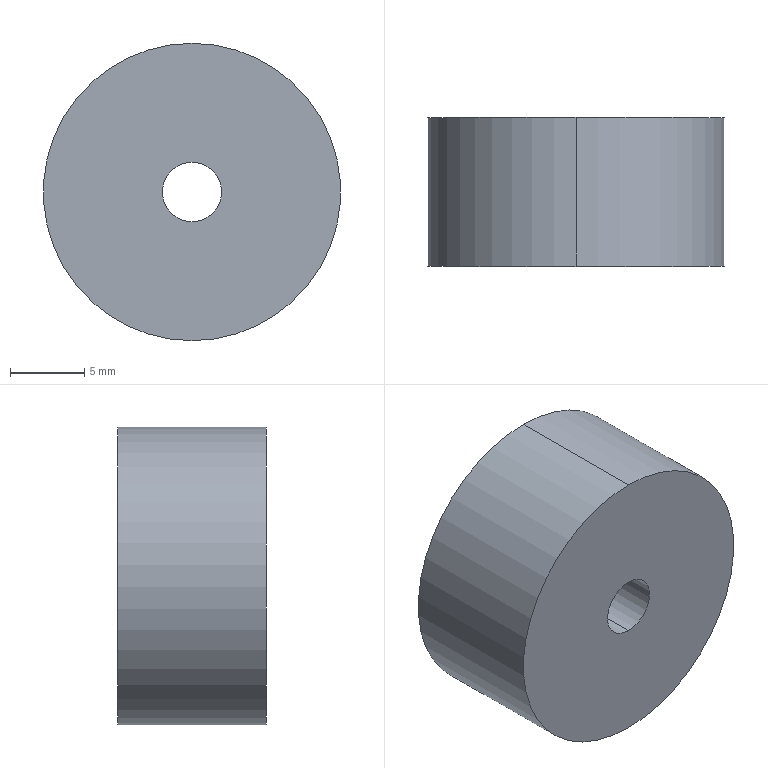Part | STEP file | 1 solid | 9 faces | box 20 x 10 x 20 mm | volume 2790 mm3 | cylinder 6 | plane 3 | commonest cylinder face diameters 4 x2 8 x2 20 x2
STEP:
#1=CARTESIAN_POINT('',(0.,0.,0.));
#2=DIRECTION('',(0.,0.,1.));
#3=DIRECTION('',(1.,0.,0.));
#4=AXIS2_PLACEMENT_3D('',#1,#2,#3);
#5=CARTESIAN_POINT('',(0.,4.,4.));
#6=VERTEX_POINT('',#5);
#7=CARTESIAN_POINT('',(0.,10.,4.));
#8=VERTEX_POINT('',#7);
#9=CARTESIAN_POINT('',(0.,10.,4.));
#10=DIRECTION('',(0.,1.,0.));
#11=VECTOR('',#10,1.);
#12=LINE('',#9,#11);
#13=CARTESIAN_POINT('',(0.,10.,0.));
#14=DIRECTION('',(0.,1.,0.));
#15=DIRECTION('',(0.,0.,1.));
#16=AXIS2_PLACEMENT_3D('',#13,#14,#15);
#17=CYLINDRICAL_SURFACE('',#16,4.);
#18=CARTESIAN_POINT('',(6.283,0.));
#19=DIRECTION('',(0.,1.));
#20=VECTOR('',#19,1.);
#21=LINE('',#18,#20);
#22=(GEOMETRIC_REPRESENTATION_CONTEXT(2)PARAMETRIC_REPRESENTATION_CONTEXT()REPRESENTATION_CONTEXT('',''));
#23=DEFINITIONAL_REPRESENTATION('',(#21),#22);
#24=PCURVE('',#17,#23);
#25=CARTESIAN_POINT('',(0.,10.,0.));
#26=DIRECTION('',(0.,1.,0.));
#27=DIRECTION('',(0.,0.,1.));
#28=AXIS2_PLACEMENT_3D('',#25,#26,#27);
#29=CYLINDRICAL_SURFACE('',#28,4.);
#30=CARTESIAN_POINT('',(0.,0.));
#31=DIRECTION('',(0.,1.));
#32=VECTOR('',#31,1.);
#33=LINE('',#30,#32);
#34=(GEOMETRIC_REPRESENTATION_CONTEXT(2)PARAMETRIC_REPRESENTATION_CONTEXT()REPRESENTATION_CONTEXT('',''));
#35=DEFINITIONAL_REPRESENTATION('',(#33),#34);
#36=PCURVE('',#29,#35);
#37=SURFACE_CURVE('',#12,(#24,#36),.PCURVE_S1.);
#38=EDGE_CURVE('',#6,#8,#37,.T.);
#39=ORIENTED_EDGE('',*,*,#38,.T.);
#40=CARTESIAN_POINT('',(0.,10.,-4.));
#41=VERTEX_POINT('',#40);
#42=CARTESIAN_POINT('',(0.,10.,0.));
#43=DIRECTION('',(0.,1.,0.));
#44=DIRECTION('',(0.,0.,1.));
#45=AXIS2_PLACEMENT_3D('',#42,#43,#44);
#46=CIRCLE('',#45,4.);
#47=CARTESIAN_POINT('',(0.,0.));
#48=DIRECTION('',(1.,0.));
#49=VECTOR('',#48,1.);
#50=LINE('',#47,#49);
#51=(GEOMETRIC_REPRESENTATION_CONTEXT(2)PARAMETRIC_REPRESENTATION_CONTEXT()REPRESENTATION_CONTEXT('',''));
#52=DEFINITIONAL_REPRESENTATION('',(#50),#51);
#53=PCURVE('',#17,#52);
#54=CARTESIAN_POINT('',(0.,10.,0.));
#55=DIRECTION('',(0.,1.,0.));
#56=DIRECTION('',(0.,0.,1.));
#57=AXIS2_PLACEMENT_3D('',#54,#55,#56);
#58=PLANE('',#57);
#59=CARTESIAN_POINT('',(0.,0.));
#60=DIRECTION('',(1.,0.));
#61=AXIS2_PLACEMENT_2D('',#59,#60);
#62=CIRCLE('',#61,4.);
#63=(GEOMETRIC_REPRESENTATION_CONTEXT(2)PARAMETRIC_REPRESENTATION_CONTEXT()REPRESENTATION_CONTEXT('',''));
#64=DEFINITIONAL_REPRESENTATION('',(#62),#63);
#65=PCURVE('',#58,#64);
#66=SURFACE_CURVE('',#46,(#53,#65),.PCURVE_S1.);
#67=EDGE_CURVE('',#41,#8,#66,.T.);
#68=ORIENTED_EDGE('',*,*,#67,.F.);
#69=CARTESIAN_POINT('',(0.,4.,-4.));
#70=VERTEX_POINT('',#69);
#71=CARTESIAN_POINT('',(0.,10.,-4.));
#72=DIRECTION('',(0.,1.,0.));
#73=VECTOR('',#72,1.);
#74=LINE('',#71,#73);
#75=CARTESIAN_POINT('',(3.142,0.));
#76=DIRECTION('',(0.,1.));
#77=VECTOR('',#76,1.);
#78=LINE('',#75,#77);
#79=(GEOMETRIC_REPRESENTATION_CONTEXT(2)PARAMETRIC_REPRESENTATION_CONTEXT()REPRESENTATION_CONTEXT('',''));
#80=DEFINITIONAL_REPRESENTATION('',(#78),#79);
#81=PCURVE('',#17,#80);
#82=CARTESIAN_POINT('',(3.142,0.));
#83=DIRECTION('',(0.,1.));
#84=VECTOR('',#83,1.);
#85=LINE('',#82,#84);
#86=(GEOMETRIC_REPRESENTATION_CONTEXT(2)PARAMETRIC_REPRESENTATION_CONTEXT()REPRESENTATION_CONTEXT('',''));
#87=DEFINITIONAL_REPRESENTATION('',(#85),#86);
#88=PCURVE('',#29,#87);
#89=SURFACE_CURVE('',#74,(#81,#88),.PCURVE_S1.);
#90=EDGE_CURVE('',#70,#41,#89,.T.);
#91=ORIENTED_EDGE('',*,*,#90,.F.);
#92=CARTESIAN_POINT('',(0.,4.,0.));
#93=DIRECTION('',(0.,1.,0.));
#94=DIRECTION('',(0.,0.,1.));
#95=AXIS2_PLACEMENT_3D('',#92,#93,#94);
#96=CIRCLE('',#95,4.);
#97=CARTESIAN_POINT('',(0.,-6.));
#98=DIRECTION('',(1.,0.));
#99=VECTOR('',#98,1.);
#100=LINE('',#97,#99);
#101=(GEOMETRIC_REPRESENTATION_CONTEXT(2)PARAMETRIC_REPRESENTATION_CONTEXT()REPRESENTATION_CONTEXT('',''));
#102=DEFINITIONAL_REPRESENTATION('',(#100),#101);
#103=PCURVE('',#17,#102);
#104=CARTESIAN_POINT('',(2.,4.,0.));
#105=DIRECTION('',(0.,-1.,0.));
#106=DIRECTION('',(0.,0.,-1.));
#107=AXIS2_PLACEMENT_3D('',#104,#105,#106);
#108=PLANE('',#107);
#109=CARTESIAN_POINT('',(-4.,-2.));
#110=CARTESIAN_POINT('',(-4.,4.928));
#111=CARTESIAN_POINT('',(2.,1.464));
#112=CARTESIAN_POINT('',(8.,-2.));
#113=CARTESIAN_POINT('',(2.,-5.464));
#114=CARTESIAN_POINT('',(-4.,-8.928));
#115=CARTESIAN_POINT('',(-4.,-2.));
#116=(BOUNDED_CURVE()B_SPLINE_CURVE(2,(#109,#110,#111,#112,#113,#114,#115),.UNSPECIFIED.,.T.,.F.)B_SPLINE_CURVE_WITH_KNOTS((1,2,2,2,2,1),(-2.094,0.,2.094,4.189,6.283,8.378),.UNSPECIFIED.)CURVE()GEOMETRIC_REPRESENTATION_ITEM()RATIONAL_B_SPLINE_CURVE((1.,0.5,1.,0.5,1.,0.5,1.))REPRESENTATION_ITEM(''));
#117=(GEOMETRIC_REPRESENTATION_CONTEXT(2)PARAMETRIC_REPRESENTATION_CONTEXT()REPRESENTATION_CONTEXT('',''));
#118=DEFINITIONAL_REPRESENTATION('',(#116),#117);
#119=PCURVE('',#108,#118);
#120=SURFACE_CURVE('',#96,(#103,#119),.PCURVE_S1.);
#121=EDGE_CURVE('',#70,#6,#120,.T.);
#122=ORIENTED_EDGE('',*,*,#121,.T.);
#123=EDGE_LOOP('',(#39,#68,#91,#122));
#124=FACE_BOUND('',#123,.F.);
#125=ADVANCED_FACE('',(#124),#17,.F.);
#126=CARTESIAN_POINT('',(0.,0.,2.));
#127=VERTEX_POINT('',#126);
#128=CARTESIAN_POINT('',(0.,4.,2.));
#129=VERTEX_POINT('',#128);
#130=CARTESIAN_POINT('',(0.,10.,2.));
#131=DIRECTION('',(0.,1.,0.));
#132=VECTOR('',#131,1.);
#133=LINE('',#130,#132);
#134=CARTESIAN_POINT('',(0.,10.,0.));
#135=DIRECTION('',(0.,1.,0.));
#136=DIRECTION('',(0.,0.,1.));
#137=AXIS2_PLACEMENT_3D('',#134,#135,#136);
#138=CYLINDRICAL_SURFACE('',#137,2.);
#139=CARTESIAN_POINT('',(6.283,0.));
#140=DIRECTION('',(0.,1.));
#141=VECTOR('',#140,1.);
#142=LINE('',#139,#141);
#143=(GEOMETRIC_REPRESENTATION_CONTEXT(2)PARAMETRIC_REPRESENTATION_CONTEXT()REPRESENTATION_CONTEXT('',''));
#144=DEFINITIONAL_REPRESENTATION('',(#142),#143);
#145=PCURVE('',#138,#144);
#146=CARTESIAN_POINT('',(0.,10.,0.));
#147=DIRECTION('',(0.,1.,0.));
#148=DIRECTION('',(0.,0.,1.));
#149=AXIS2_PLACEMENT_3D('',#146,#147,#148);
#150=CYLINDRICAL_SURFACE('',#149,2.);
#151=CARTESIAN_POINT('',(0.,0.));
#152=DIRECTION('',(0.,1.));
#153=VECTOR('',#152,1.);
#154=LINE('',#151,#153);
#155=(GEOMETRIC_REPRESENTATION_CONTEXT(2)PARAMETRIC_REPRESENTATION_CONTEXT()REPRESENTATION_CONTEXT('',''));
#156=DEFINITIONAL_REPRESENTATION('',(#154),#155);
#157=PCURVE('',#150,#156);
#158=SURFACE_CURVE('',#133,(#145,#157),.PCURVE_S1.);
#159=EDGE_CURVE('',#127,#129,#158,.T.);
#160=ORIENTED_EDGE('',*,*,#159,.T.);
#161=CARTESIAN_POINT('',(0.,4.,-2.));
#162=VERTEX_POINT('',#161);
#163=CARTESIAN_POINT('',(0.,4.,0.));
#164=DIRECTION('',(0.,1.,0.));
#165=DIRECTION('',(0.,0.,1.));
#166=AXIS2_PLACEMENT_3D('',#163,#164,#165);
#167=CIRCLE('',#166,2.);
#168=CARTESIAN_POINT('',(0.,-6.));
#169=DIRECTION('',(1.,0.));
#170=VECTOR('',#169,1.);
#171=LINE('',#168,#170);
#172=(GEOMETRIC_REPRESENTATION_CONTEXT(2)PARAMETRIC_REPRESENTATION_CONTEXT()REPRESENTATION_CONTEXT('',''));
#173=DEFINITIONAL_REPRESENTATION('',(#171),#172);
#174=PCURVE('',#138,#173);
#175=CARTESIAN_POINT('',(-2.,-2.));
#176=CARTESIAN_POINT('',(-2.,1.464));
#177=CARTESIAN_POINT('',(1.,-0.2679));
#178=CARTESIAN_POINT('',(4.,-2.));
#179=CARTESIAN_POINT('',(1.,-3.732));
#180=CARTESIAN_POINT('',(-2.,-5.464));
#181=CARTESIAN_POINT('',(-2.,-2.));
#182=(BOUNDED_CURVE()B_SPLINE_CURVE(2,(#175,#176,#177,#178,#179,#180,#181),.UNSPECIFIED.,.T.,.F.)B_SPLINE_CURVE_WITH_KNOTS((1,2,2,2,2,1),(-2.094,0.,2.094,4.189,6.283,8.378),.UNSPECIFIED.)CURVE()GEOMETRIC_REPRESENTATION_ITEM()RATIONAL_B_SPLINE_CURVE((1.,0.5,1.,0.5,1.,0.5,1.))REPRESENTATION_ITEM(''));
#183=(GEOMETRIC_REPRESENTATION_CONTEXT(2)PARAMETRIC_REPRESENTATION_CONTEXT()REPRESENTATION_CONTEXT('',''));
#184=DEFINITIONAL_REPRESENTATION('',(#182),#183);
#185=PCURVE('',#108,#184);
#186=SURFACE_CURVE('',#167,(#174,#185),.PCURVE_S1.);
#187=EDGE_CURVE('',#162,#129,#186,.T.);
#188=ORIENTED_EDGE('',*,*,#187,.F.);
#189=CARTESIAN_POINT('',(0.,0.,-2.));
#190=VERTEX_POINT('',#189);
#191=CARTESIAN_POINT('',(0.,10.,-2.));
#192=DIRECTION('',(0.,1.,0.));
#193=VECTOR('',#192,1.);
#194=LINE('',#191,#193);
#195=CARTESIAN_POINT('',(3.142,0.));
#196=DIRECTION('',(0.,1.));
#197=VECTOR('',#196,1.);
#198=LINE('',#195,#197);
#199=(GEOMETRIC_REPRESENTATION_CONTEXT(2)PARAMETRIC_REPRESENTATION_CONTEXT()REPRESENTATION_CONTEXT('',''));
#200=DEFINITIONAL_REPRESENTATION('',(#198),#199);
#201=PCURVE('',#138,#200);
#202=CARTESIAN_POINT('',(3.142,0.));
#203=DIRECTION('',(0.,1.));
#204=VECTOR('',#203,1.);
#205=LINE('',#202,#204);
#206=(GEOMETRIC_REPRESENTATION_CONTEXT(2)PARAMETRIC_REPRESENTATION_CONTEXT()REPRESENTATION_CONTEXT('',''));
#207=DEFINITIONAL_REPRESENTATION('',(#205),#206);
#208=PCURVE('',#150,#207);
#209=SURFACE_CURVE('',#194,(#201,#208),.PCURVE_S1.);
#210=EDGE_CURVE('',#190,#162,#209,.T.);
#211=ORIENTED_EDGE('',*,*,#210,.F.);
#212=CARTESIAN_POINT('',(0.,0.,0.));
#213=DIRECTION('',(0.,1.,0.));
#214=DIRECTION('',(0.,0.,1.));
#215=AXIS2_PLACEMENT_3D('',#212,#213,#214);
#216=CIRCLE('',#215,2.);
#217=CARTESIAN_POINT('',(0.,-10.));
#218=DIRECTION('',(1.,0.));
#219=VECTOR('',#218,1.);
#220=LINE('',#217,#219);
#221=(GEOMETRIC_REPRESENTATION_CONTEXT(2)PARAMETRIC_REPRESENTATION_CONTEXT()REPRESENTATION_CONTEXT('',''));
#222=DEFINITIONAL_REPRESENTATION('',(#220),#221);
#223=PCURVE('',#138,#222);
#224=CARTESIAN_POINT('',(0.,0.,0.));
#225=DIRECTION('',(0.,1.,0.));
#226=DIRECTION('',(0.,0.,1.));
#227=AXIS2_PLACEMENT_3D('',#224,#225,#226);
#228=PLANE('',#227);
#229=CARTESIAN_POINT('',(0.,0.));
#230=DIRECTION('',(1.,0.));
#231=AXIS2_PLACEMENT_2D('',#229,#230);
#232=CIRCLE('',#231,2.);
#233=(GEOMETRIC_REPRESENTATION_CONTEXT(2)PARAMETRIC_REPRESENTATION_CONTEXT()REPRESENTATION_CONTEXT('',''));
#234=DEFINITIONAL_REPRESENTATION('',(#232),#233);
#235=PCURVE('',#228,#234);
#236=SURFACE_CURVE('',#216,(#223,#235),.PCURVE_S1.);
#237=EDGE_CURVE('',#190,#127,#236,.T.);
#238=ORIENTED_EDGE('',*,*,#237,.T.);
#239=EDGE_LOOP('',(#160,#188,#211,#238));
#240=FACE_BOUND('',#239,.F.);
#241=ADVANCED_FACE('',(#240),#138,.F.);
#242=CARTESIAN_POINT('',(0.,10.,10.));
#243=VERTEX_POINT('',#242);
#244=CARTESIAN_POINT('',(0.,10.,-10.));
#245=VERTEX_POINT('',#244);
#246=CARTESIAN_POINT('',(0.,10.,0.));
#247=DIRECTION('',(0.,1.,0.));
#248=DIRECTION('',(0.,0.,1.));
#249=AXIS2_PLACEMENT_3D('',#246,#247,#248);
#250=CIRCLE('',#249,10.);
#251=CARTESIAN_POINT('',(0.,10.,0.));
#252=DIRECTION('',(0.,-1.,0.));
#253=DIRECTION('',(0.,0.,-1.));
#254=AXIS2_PLACEMENT_3D('',#251,#252,#253);
#255=CYLINDRICAL_SURFACE('',#254,10.);
#256=CARTESIAN_POINT('',(3.142,0.));
#257=DIRECTION('',(-1.,0.));
#258=VECTOR('',#257,1.);
#259=LINE('',#256,#258);
#260=(GEOMETRIC_REPRESENTATION_CONTEXT(2)PARAMETRIC_REPRESENTATION_CONTEXT()REPRESENTATION_CONTEXT('',''));
#261=DEFINITIONAL_REPRESENTATION('',(#259),#260);
#262=PCURVE('',#255,#261);
#263=CARTESIAN_POINT('',(0.,0.));
#264=DIRECTION('',(1.,0.));
#265=AXIS2_PLACEMENT_2D('',#263,#264);
#266=CIRCLE('',#265,10.);
#267=(GEOMETRIC_REPRESENTATION_CONTEXT(2)PARAMETRIC_REPRESENTATION_CONTEXT()REPRESENTATION_CONTEXT('',''));
#268=DEFINITIONAL_REPRESENTATION('',(#266),#267);
#269=PCURVE('',#58,#268);
#270=SURFACE_CURVE('',#250,(#262,#269),.PCURVE_S1.);
#271=EDGE_CURVE('',#243,#245,#270,.T.);
#272=ORIENTED_EDGE('',*,*,#271,.F.);
#273=CARTESIAN_POINT('',(0.,0.,10.));
#274=VERTEX_POINT('',#273);
#275=CARTESIAN_POINT('',(0.,10.,10.));
#276=DIRECTION('',(0.,-1.,0.));
#277=VECTOR('',#276,1.);
#278=LINE('',#275,#277);
#279=CARTESIAN_POINT('',(3.142,0.));
#280=DIRECTION('',(0.,1.));
#281=VECTOR('',#280,1.);
#282=LINE('',#279,#281);
#283=(GEOMETRIC_REPRESENTATION_CONTEXT(2)PARAMETRIC_REPRESENTATION_CONTEXT()REPRESENTATION_CONTEXT('',''));
#284=DEFINITIONAL_REPRESENTATION('',(#282),#283);
#285=PCURVE('',#255,#284);
#286=CARTESIAN_POINT('',(0.,10.,0.));
#287=DIRECTION('',(0.,-1.,0.));
#288=DIRECTION('',(0.,0.,-1.));
#289=AXIS2_PLACEMENT_3D('',#286,#287,#288);
#290=CYLINDRICAL_SURFACE('',#289,10.);
#291=CARTESIAN_POINT('',(3.142,0.));
#292=DIRECTION('',(0.,1.));
#293=VECTOR('',#292,1.);
#294=LINE('',#291,#293);
#295=(GEOMETRIC_REPRESENTATION_CONTEXT(2)PARAMETRIC_REPRESENTATION_CONTEXT()REPRESENTATION_CONTEXT('',''));
#296=DEFINITIONAL_REPRESENTATION('',(#294),#295);
#297=PCURVE('',#290,#296);
#298=SURFACE_CURVE('',#278,(#285,#297),.PCURVE_S1.);
#299=EDGE_CURVE('',#243,#274,#298,.T.);
#300=ORIENTED_EDGE('',*,*,#299,.T.);
#301=CARTESIAN_POINT('',(0.,0.,-10.));
#302=VERTEX_POINT('',#301);
#303=CARTESIAN_POINT('',(0.,0.,0.));
#304=DIRECTION('',(0.,1.,0.));
#305=DIRECTION('',(0.,0.,1.));
#306=AXIS2_PLACEMENT_3D('',#303,#304,#305);
#307=CIRCLE('',#306,10.);
#308=CARTESIAN_POINT('',(3.142,10.));
#309=DIRECTION('',(-1.,0.));
#310=VECTOR('',#309,1.);
#311=LINE('',#308,#310);
#312=(GEOMETRIC_REPRESENTATION_CONTEXT(2)PARAMETRIC_REPRESENTATION_CONTEXT()REPRESENTATION_CONTEXT('',''));
#313=DEFINITIONAL_REPRESENTATION('',(#311),#312);
#314=PCURVE('',#255,#313);
#315=CARTESIAN_POINT('',(0.,0.));
#316=DIRECTION('',(1.,0.));
#317=AXIS2_PLACEMENT_2D('',#315,#316);
#318=CIRCLE('',#317,10.);
#319=(GEOMETRIC_REPRESENTATION_CONTEXT(2)PARAMETRIC_REPRESENTATION_CONTEXT()REPRESENTATION_CONTEXT('',''));
#320=DEFINITIONAL_REPRESENTATION('',(#318),#319);
#321=PCURVE('',#228,#320);
#322=SURFACE_CURVE('',#307,(#314,#321),.PCURVE_S1.);
#323=EDGE_CURVE('',#274,#302,#322,.T.);
#324=ORIENTED_EDGE('',*,*,#323,.T.);
#325=CARTESIAN_POINT('',(0.,10.,-10.));
#326=DIRECTION('',(0.,-1.,0.));
#327=VECTOR('',#326,1.);
#328=LINE('',#325,#327);
#329=CARTESIAN_POINT('',(0.,0.));
#330=DIRECTION('',(0.,1.));
#331=VECTOR('',#330,1.);
#332=LINE('',#329,#331);
#333=(GEOMETRIC_REPRESENTATION_CONTEXT(2)PARAMETRIC_REPRESENTATION_CONTEXT()REPRESENTATION_CONTEXT('',''));
#334=DEFINITIONAL_REPRESENTATION('',(#332),#333);
#335=PCURVE('',#255,#334);
#336=CARTESIAN_POINT('',(6.283,0.));
#337=DIRECTION('',(0.,1.));
#338=VECTOR('',#337,1.);
#339=LINE('',#336,#338);
#340=(GEOMETRIC_REPRESENTATION_CONTEXT(2)PARAMETRIC_REPRESENTATION_CONTEXT()REPRESENTATION_CONTEXT('',''));
#341=DEFINITIONAL_REPRESENTATION('',(#339),#340);
#342=PCURVE('',#290,#341);
#343=SURFACE_CURVE('',#328,(#335,#342),.PCURVE_S1.);
#344=EDGE_CURVE('',#245,#302,#343,.T.);
#345=ORIENTED_EDGE('',*,*,#344,.F.);
#346=EDGE_LOOP('',(#272,#300,#324,#345));
#347=FACE_BOUND('',#346,.T.);
#348=ADVANCED_FACE('',(#347),#255,.T.);
#349=ORIENTED_EDGE('',*,*,#299,.F.);
#350=CARTESIAN_POINT('',(0.,10.,0.));
#351=DIRECTION('',(0.,1.,0.));
#352=DIRECTION('',(0.,0.,1.));
#353=AXIS2_PLACEMENT_3D('',#350,#351,#352);
#354=CIRCLE('',#353,10.);
#355=CARTESIAN_POINT('',(9.425,0.));
#356=DIRECTION('',(-1.,0.));
#357=VECTOR('',#356,1.);
#358=LINE('',#355,#357);
#359=(GEOMETRIC_REPRESENTATION_CONTEXT(2)PARAMETRIC_REPRESENTATION_CONTEXT()REPRESENTATION_CONTEXT('',''));
#360=DEFINITIONAL_REPRESENTATION('',(#358),#359);
#361=PCURVE('',#290,#360);
#362=CARTESIAN_POINT('',(0.,0.));
#363=DIRECTION('',(1.,0.));
#364=AXIS2_PLACEMENT_2D('',#362,#363);
#365=CIRCLE('',#364,10.);
#366=(GEOMETRIC_REPRESENTATION_CONTEXT(2)PARAMETRIC_REPRESENTATION_CONTEXT()REPRESENTATION_CONTEXT('',''));
#367=DEFINITIONAL_REPRESENTATION('',(#365),#366);
#368=PCURVE('',#58,#367);
#369=SURFACE_CURVE('',#354,(#361,#368),.PCURVE_S1.);
#370=EDGE_CURVE('',#245,#243,#369,.T.);
#371=ORIENTED_EDGE('',*,*,#370,.F.);
#372=ORIENTED_EDGE('',*,*,#344,.T.);
#373=CARTESIAN_POINT('',(0.,0.,0.));
#374=DIRECTION('',(0.,1.,0.));
#375=DIRECTION('',(0.,0.,1.));
#376=AXIS2_PLACEMENT_3D('',#373,#374,#375);
#377=CIRCLE('',#376,10.);
#378=CARTESIAN_POINT('',(9.425,10.));
#379=DIRECTION('',(-1.,0.));
#380=VECTOR('',#379,1.);
#381=LINE('',#378,#380);
#382=(GEOMETRIC_REPRESENTATION_CONTEXT(2)PARAMETRIC_REPRESENTATION_CONTEXT()REPRESENTATION_CONTEXT('',''));
#383=DEFINITIONAL_REPRESENTATION('',(#381),#382);
#384=PCURVE('',#290,#383);
#385=CARTESIAN_POINT('',(0.,0.));
#386=DIRECTION('',(1.,0.));
#387=AXIS2_PLACEMENT_2D('',#385,#386);
#388=CIRCLE('',#387,10.);
#389=(GEOMETRIC_REPRESENTATION_CONTEXT(2)PARAMETRIC_REPRESENTATION_CONTEXT()REPRESENTATION_CONTEXT('',''));
#390=DEFINITIONAL_REPRESENTATION('',(#388),#389);
#391=PCURVE('',#228,#390);
#392=SURFACE_CURVE('',#377,(#384,#391),.PCURVE_S1.);
#393=EDGE_CURVE('',#302,#274,#392,.T.);
#394=ORIENTED_EDGE('',*,*,#393,.T.);
#395=EDGE_LOOP('',(#349,#371,#372,#394));
#396=FACE_BOUND('',#395,.T.);
#397=ADVANCED_FACE('',(#396),#290,.T.);
#398=CARTESIAN_POINT('',(0.,10.,0.));
#399=DIRECTION('',(0.,1.,0.));
#400=DIRECTION('',(0.,0.,1.));
#401=AXIS2_PLACEMENT_3D('',#398,#399,#400);
#402=CIRCLE('',#401,4.);
#403=CARTESIAN_POINT('',(0.,0.));
#404=DIRECTION('',(1.,0.));
#405=AXIS2_PLACEMENT_2D('',#403,#404);
#406=CIRCLE('',#405,4.);
#407=(GEOMETRIC_REPRESENTATION_CONTEXT(2)PARAMETRIC_REPRESENTATION_CONTEXT()REPRESENTATION_CONTEXT('',''));
#408=DEFINITIONAL_REPRESENTATION('',(#406),#407);
#409=PCURVE('',#58,#408);
#410=CARTESIAN_POINT('',(0.,0.));
#411=DIRECTION('',(1.,0.));
#412=VECTOR('',#411,1.);
#413=LINE('',#410,#412);
#414=(GEOMETRIC_REPRESENTATION_CONTEXT(2)PARAMETRIC_REPRESENTATION_CONTEXT()REPRESENTATION_CONTEXT('',''));
#415=DEFINITIONAL_REPRESENTATION('',(#413),#414);
#416=PCURVE('',#29,#415);
#417=SURFACE_CURVE('',#402,(#409,#416),.PCURVE_S1.);
#418=EDGE_CURVE('',#8,#41,#417,.T.);
#419=ORIENTED_EDGE('',*,*,#418,.F.);
#420=ORIENTED_EDGE('',*,*,#67,.F.);
#421=EDGE_LOOP('',(#419,#420));
#422=FACE_BOUND('',#421,.T.);
#423=ORIENTED_EDGE('',*,*,#370,.T.);
#424=ORIENTED_EDGE('',*,*,#271,.T.);
#425=EDGE_LOOP('',(#423,#424));
#426=FACE_BOUND('',#425,.T.);
#427=ADVANCED_FACE('',(#422,#426),#58,.T.);
#428=CARTESIAN_POINT('',(0.,0.,0.));
#429=DIRECTION('',(0.,1.,0.));
#430=DIRECTION('',(0.,0.,1.));
#431=AXIS2_PLACEMENT_3D('',#428,#429,#430);
#432=CIRCLE('',#431,2.);
#433=CARTESIAN_POINT('',(0.,0.));
#434=DIRECTION('',(1.,0.));
#435=AXIS2_PLACEMENT_2D('',#433,#434);
#436=CIRCLE('',#435,2.);
#437=(GEOMETRIC_REPRESENTATION_CONTEXT(2)PARAMETRIC_REPRESENTATION_CONTEXT()REPRESENTATION_CONTEXT('',''));
#438=DEFINITIONAL_REPRESENTATION('',(#436),#437);
#439=PCURVE('',#228,#438);
#440=CARTESIAN_POINT('',(0.,-10.));
#441=DIRECTION('',(1.,0.));
#442=VECTOR('',#441,1.);
#443=LINE('',#440,#442);
#444=(GEOMETRIC_REPRESENTATION_CONTEXT(2)PARAMETRIC_REPRESENTATION_CONTEXT()REPRESENTATION_CONTEXT('',''));
#445=DEFINITIONAL_REPRESENTATION('',(#443),#444);
#446=PCURVE('',#150,#445);
#447=SURFACE_CURVE('',#432,(#439,#446),.PCURVE_S1.);
#448=EDGE_CURVE('',#127,#190,#447,.T.);
#449=ORIENTED_EDGE('',*,*,#448,.T.);
#450=ORIENTED_EDGE('',*,*,#237,.T.);
#451=EDGE_LOOP('',(#449,#450));
#452=FACE_BOUND('',#451,.T.);
#453=ORIENTED_EDGE('',*,*,#393,.F.);
#454=ORIENTED_EDGE('',*,*,#323,.F.);
#455=EDGE_LOOP('',(#453,#454));
#456=FACE_BOUND('',#455,.T.);
#457=ADVANCED_FACE('',(#452,#456),#228,.F.);
#458=CARTESIAN_POINT('',(0.,4.,0.));
#459=DIRECTION('',(0.,1.,0.));
#460=DIRECTION('',(0.,0.,1.));
#461=AXIS2_PLACEMENT_3D('',#458,#459,#460);
#462=CIRCLE('',#461,2.);
#463=CARTESIAN_POINT('',(0.,-6.));
#464=DIRECTION('',(1.,0.));
#465=VECTOR('',#464,1.);
#466=LINE('',#463,#465);
#467=(GEOMETRIC_REPRESENTATION_CONTEXT(2)PARAMETRIC_REPRESENTATION_CONTEXT()REPRESENTATION_CONTEXT('',''));
#468=DEFINITIONAL_REPRESENTATION('',(#466),#467);
#469=PCURVE('',#150,#468);
#470=CARTESIAN_POINT('',(-2.,-2.));
#471=CARTESIAN_POINT('',(-2.,1.464));
#472=CARTESIAN_POINT('',(1.,-0.2679));
#473=CARTESIAN_POINT('',(4.,-2.));
#474=CARTESIAN_POINT('',(1.,-3.732));
#475=CARTESIAN_POINT('',(-2.,-5.464));
#476=CARTESIAN_POINT('',(-2.,-2.));
#477=(BOUNDED_CURVE()B_SPLINE_CURVE(2,(#470,#471,#472,#473,#474,#475,#476),.UNSPECIFIED.,.T.,.F.)B_SPLINE_CURVE_WITH_KNOTS((1,2,2,2,2,1),(-2.094,0.,2.094,4.189,6.283,8.378),.UNSPECIFIED.)CURVE()GEOMETRIC_REPRESENTATION_ITEM()RATIONAL_B_SPLINE_CURVE((1.,0.5,1.,0.5,1.,0.5,1.))REPRESENTATION_ITEM(''));
#478=(GEOMETRIC_REPRESENTATION_CONTEXT(2)PARAMETRIC_REPRESENTATION_CONTEXT()REPRESENTATION_CONTEXT('',''));
#479=DEFINITIONAL_REPRESENTATION('',(#477),#478);
#480=PCURVE('',#108,#479);
#481=SURFACE_CURVE('',#462,(#469,#480),.PCURVE_S1.);
#482=EDGE_CURVE('',#129,#162,#481,.T.);
#483=ORIENTED_EDGE('',*,*,#482,.F.);
#484=ORIENTED_EDGE('',*,*,#159,.F.);
#485=ORIENTED_EDGE('',*,*,#448,.T.);
#486=ORIENTED_EDGE('',*,*,#210,.T.);
#487=EDGE_LOOP('',(#483,#484,#485,#486));
#488=FACE_BOUND('',#487,.F.);
#489=ADVANCED_FACE('',(#488),#150,.F.);
#490=ORIENTED_EDGE('',*,*,#482,.F.);
#491=ORIENTED_EDGE('',*,*,#187,.F.);
#492=EDGE_LOOP('',(#490,#491));
#493=FACE_BOUND('',#492,.T.);
#494=CARTESIAN_POINT('',(0.,4.,0.));
#495=DIRECTION('',(0.,1.,0.));
#496=DIRECTION('',(0.,0.,1.));
#497=AXIS2_PLACEMENT_3D('',#494,#495,#496);
#498=CIRCLE('',#497,4.);
#499=CARTESIAN_POINT('',(-4.,-2.));
#500=CARTESIAN_POINT('',(-4.,4.928));
#501=CARTESIAN_POINT('',(2.,1.464));
#502=CARTESIAN_POINT('',(8.,-2.));
#503=CARTESIAN_POINT('',(2.,-5.464));
#504=CARTESIAN_POINT('',(-4.,-8.928));
#505=CARTESIAN_POINT('',(-4.,-2.));
#506=(BOUNDED_CURVE()B_SPLINE_CURVE(2,(#499,#500,#501,#502,#503,#504,#505),.UNSPECIFIED.,.T.,.F.)B_SPLINE_CURVE_WITH_KNOTS((1,2,2,2,2,1),(-2.094,0.,2.094,4.189,6.283,8.378),.UNSPECIFIED.)CURVE()GEOMETRIC_REPRESENTATION_ITEM()RATIONAL_B_SPLINE_CURVE((1.,0.5,1.,0.5,1.,0.5,1.))REPRESENTATION_ITEM(''));
#507=(GEOMETRIC_REPRESENTATION_CONTEXT(2)PARAMETRIC_REPRESENTATION_CONTEXT()REPRESENTATION_CONTEXT('',''));
#508=DEFINITIONAL_REPRESENTATION('',(#506),#507);
#509=PCURVE('',#108,#508);
#510=CARTESIAN_POINT('',(0.,-6.));
#511=DIRECTION('',(1.,0.));
#512=VECTOR('',#511,1.);
#513=LINE('',#510,#512);
#514=(GEOMETRIC_REPRESENTATION_CONTEXT(2)PARAMETRIC_REPRESENTATION_CONTEXT()REPRESENTATION_CONTEXT('',''));
#515=DEFINITIONAL_REPRESENTATION('',(#513),#514);
#516=PCURVE('',#29,#515);
#517=SURFACE_CURVE('',#498,(#509,#516),.PCURVE_S1.);
#518=EDGE_CURVE('',#6,#70,#517,.T.);
#519=ORIENTED_EDGE('',*,*,#518,.T.);
#520=ORIENTED_EDGE('',*,*,#121,.T.);
#521=EDGE_LOOP('',(#519,#520));
#522=FACE_BOUND('',#521,.T.);
#523=ADVANCED_FACE('',(#493,#522),#108,.F.);
#524=ORIENTED_EDGE('',*,*,#418,.F.);
#525=ORIENTED_EDGE('',*,*,#38,.F.);
#526=ORIENTED_EDGE('',*,*,#518,.T.);
#527=ORIENTED_EDGE('',*,*,#90,.T.);
#528=EDGE_LOOP('',(#524,#525,#526,#527));
#529=FACE_BOUND('',#528,.F.);
#530=ADVANCED_FACE('',(#529),#29,.F.);
#531=CLOSED_SHELL('',(#125,#241,#348,#397,#427,#457,#489,#523,#530));
#532=MANIFOLD_SOLID_BREP('',#531);
#533=(LENGTH_UNIT()NAMED_UNIT(*)SI_UNIT(.MILLI.,.METRE.));
#534=UNCERTAINTY_MEASURE_WITH_UNIT(LENGTH_MEASURE(0.0000001),#533,'','');
#535=(NAMED_UNIT(*)PLANE_ANGLE_UNIT()SI_UNIT($,.RADIAN.));
#536=(NAMED_UNIT(*)SI_UNIT($,.STERADIAN.)SOLID_ANGLE_UNIT());
#537=(GEOMETRIC_REPRESENTATION_CONTEXT(3)GLOBAL_UNCERTAINTY_ASSIGNED_CONTEXT((#534))GLOBAL_UNIT_ASSIGNED_CONTEXT((#533,#535,#536))REPRESENTATION_CONTEXT('',''));
#538=ADVANCED_BREP_SHAPE_REPRESENTATION('',(#4,#532),#537);